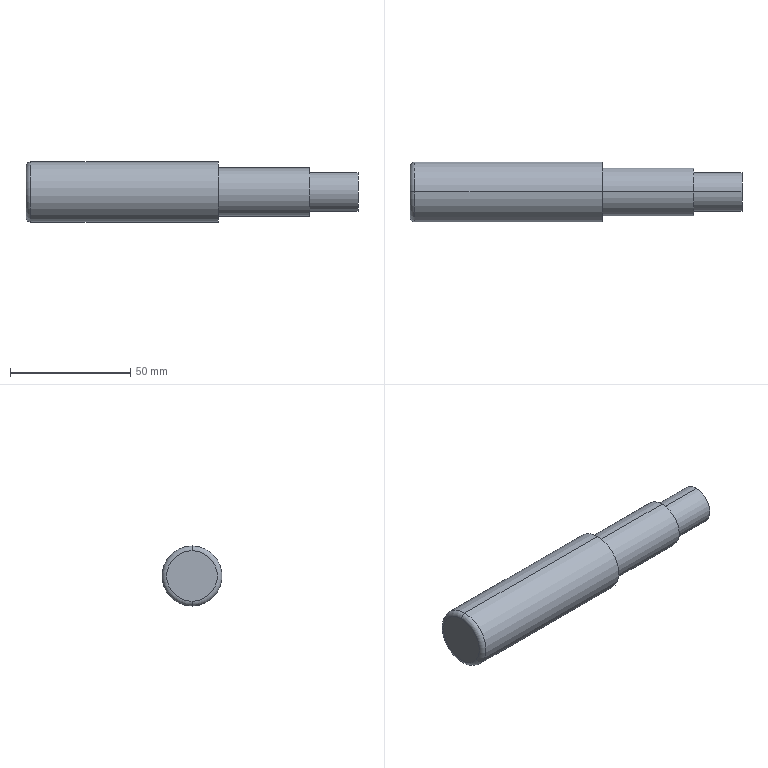Part | SolidWorks | features Fillet 1, Revolution 1 | 1 solid | 12 faces | box 138 x 25 x 25 mm | volume 55164 mm3 | cylinder 6 | plane 4 | torus 2 | commonest cylinder face diameters 16 x2 20 x2 25 x2
STEP:
#1=CARTESIAN_POINT('',(0.,0.,10.5));
#2=VERTEX_POINT('',#1);
#3=CARTESIAN_POINT('',(0.,0.,-10.5));
#4=VERTEX_POINT('',#3);
#5=CARTESIAN_POINT('',(0.,0.,0.));
#6=DIRECTION('',(-1.,0.,0.));
#7=DIRECTION('',(0.,0.,-1.));
#8=AXIS2_PLACEMENT_3D('',#5,#6,#7);
#9=CIRCLE('',#8,10.5);
#10=EDGE_CURVE('',#2,#4,#9,.T.);
#11=ORIENTED_EDGE('',*,*,#10,.F.);
#12=CARTESIAN_POINT('',(2.,0.,12.5));
#13=VERTEX_POINT('',#12);
#14=CARTESIAN_POINT('',(2.,0.,10.5));
#15=DIRECTION('',(0.,1.,0.));
#16=DIRECTION('',(0.,0.,1.));
#17=AXIS2_PLACEMENT_3D('',#14,#15,#16);
#18=CIRCLE('',#17,2.);
#19=EDGE_CURVE('',#2,#13,#18,.T.);
#20=ORIENTED_EDGE('',*,*,#19,.T.);
#21=CARTESIAN_POINT('',(2.,0.,-12.5));
#22=VERTEX_POINT('',#21);
#23=CARTESIAN_POINT('',(2.,0.,0.));
#24=DIRECTION('',(1.,0.,0.));
#25=DIRECTION('',(0.,0.,-1.));
#26=AXIS2_PLACEMENT_3D('',#23,#24,#25);
#27=CIRCLE('',#26,12.5);
#28=EDGE_CURVE('',#22,#13,#27,.T.);
#29=ORIENTED_EDGE('',*,*,#28,.F.);
#30=CARTESIAN_POINT('',(2.,0.,-10.5));
#31=DIRECTION('',(0.,-1.,0.));
#32=DIRECTION('',(0.,0.,-1.));
#33=AXIS2_PLACEMENT_3D('',#30,#31,#32);
#34=CIRCLE('',#33,2.);
#35=EDGE_CURVE('',#4,#22,#34,.T.);
#36=ORIENTED_EDGE('',*,*,#35,.F.);
#37=EDGE_LOOP('',(#11,#20,#29,#36));
#38=FACE_OUTER_BOUND('',#37,.T.);
#39=CARTESIAN_POINT('',(2.,0.,0.));
#40=DIRECTION('',(1.,0.,0.));
#41=DIRECTION('',(0.,0.,-1.));
#42=AXIS2_PLACEMENT_3D('',#39,#40,#41);
#43=TOROIDAL_SURFACE('',#42,10.5,2.);
#44=ADVANCED_FACE('',(#38),#43,.T.);
#45=CARTESIAN_POINT('',(138.,0.,8.));
#46=VERTEX_POINT('',#45);
#47=CARTESIAN_POINT('',(138.,0.,-8.));
#48=VERTEX_POINT('',#47);
#49=CARTESIAN_POINT('',(138.,0.,0.));
#50=DIRECTION('',(-1.,0.,0.));
#51=DIRECTION('',(0.,0.,1.));
#52=AXIS2_PLACEMENT_3D('',#49,#50,#51);
#53=CIRCLE('',#52,8.);
#54=EDGE_CURVE('',#46,#48,#53,.T.);
#55=ORIENTED_EDGE('',*,*,#54,.T.);
#56=CARTESIAN_POINT('',(118.,0.,-8.));
#57=VERTEX_POINT('',#56);
#58=CARTESIAN_POINT('',(0.,0.,-8.));
#59=DIRECTION('',(-1.,0.,0.));
#60=VECTOR('',#59,1000.);
#61=LINE('',#58,#60);
#62=EDGE_CURVE('',#48,#57,#61,.T.);
#63=ORIENTED_EDGE('',*,*,#62,.T.);
#64=CARTESIAN_POINT('',(118.,0.,8.));
#65=VERTEX_POINT('',#64);
#66=CARTESIAN_POINT('',(118.,0.,0.));
#67=DIRECTION('',(-1.,0.,0.));
#68=DIRECTION('',(0.,0.,1.));
#69=AXIS2_PLACEMENT_3D('',#66,#67,#68);
#70=CIRCLE('',#69,8.);
#71=EDGE_CURVE('',#65,#57,#70,.T.);
#72=ORIENTED_EDGE('',*,*,#71,.F.);
#73=CARTESIAN_POINT('',(0.,0.,8.));
#74=DIRECTION('',(-1.,0.,0.));
#75=VECTOR('',#74,1000.);
#76=LINE('',#73,#75);
#77=EDGE_CURVE('',#46,#65,#76,.T.);
#78=ORIENTED_EDGE('',*,*,#77,.F.);
#79=EDGE_LOOP('',(#55,#63,#72,#78));
#80=FACE_OUTER_BOUND('',#79,.T.);
#81=CARTESIAN_POINT('',(0.,0.,0.));
#82=DIRECTION('',(-1.,0.,0.));
#83=DIRECTION('',(0.,0.,1.));
#84=AXIS2_PLACEMENT_3D('',#81,#82,#83);
#85=CYLINDRICAL_SURFACE('',#84,8.);
#86=ADVANCED_FACE('',(#80),#85,.T.);
#87=CARTESIAN_POINT('',(118.,0.,10.));
#88=VERTEX_POINT('',#87);
#89=CARTESIAN_POINT('',(118.,0.,-10.));
#90=VERTEX_POINT('',#89);
#91=CARTESIAN_POINT('',(118.,0.,0.));
#92=DIRECTION('',(-1.,0.,0.));
#93=DIRECTION('',(0.,0.,1.));
#94=AXIS2_PLACEMENT_3D('',#91,#92,#93);
#95=CIRCLE('',#94,10.);
#96=EDGE_CURVE('',#88,#90,#95,.T.);
#97=ORIENTED_EDGE('',*,*,#96,.T.);
#98=CARTESIAN_POINT('',(80.,0.,-10.));
#99=VERTEX_POINT('',#98);
#100=CARTESIAN_POINT('',(0.,0.,-10.));
#101=DIRECTION('',(-1.,0.,0.));
#102=VECTOR('',#101,1000.);
#103=LINE('',#100,#102);
#104=EDGE_CURVE('',#90,#99,#103,.T.);
#105=ORIENTED_EDGE('',*,*,#104,.T.);
#106=CARTESIAN_POINT('',(80.,0.,10.));
#107=VERTEX_POINT('',#106);
#108=CARTESIAN_POINT('',(80.,0.,0.));
#109=DIRECTION('',(-1.,0.,0.));
#110=DIRECTION('',(0.,0.,1.));
#111=AXIS2_PLACEMENT_3D('',#108,#109,#110);
#112=CIRCLE('',#111,10.);
#113=EDGE_CURVE('',#107,#99,#112,.T.);
#114=ORIENTED_EDGE('',*,*,#113,.F.);
#115=CARTESIAN_POINT('',(0.,0.,10.));
#116=DIRECTION('',(-1.,0.,0.));
#117=VECTOR('',#116,1000.);
#118=LINE('',#115,#117);
#119=EDGE_CURVE('',#88,#107,#118,.T.);
#120=ORIENTED_EDGE('',*,*,#119,.F.);
#121=EDGE_LOOP('',(#97,#105,#114,#120));
#122=FACE_OUTER_BOUND('',#121,.T.);
#123=CARTESIAN_POINT('',(0.,0.,0.));
#124=DIRECTION('',(-1.,0.,0.));
#125=DIRECTION('',(0.,0.,1.));
#126=AXIS2_PLACEMENT_3D('',#123,#124,#125);
#127=CYLINDRICAL_SURFACE('',#126,10.);
#128=ADVANCED_FACE('',(#122),#127,.T.);
#129=CARTESIAN_POINT('',(80.,0.,12.5));
#130=VERTEX_POINT('',#129);
#131=CARTESIAN_POINT('',(80.,0.,-12.5));
#132=VERTEX_POINT('',#131);
#133=CARTESIAN_POINT('',(80.,0.,0.));
#134=DIRECTION('',(-1.,0.,0.));
#135=DIRECTION('',(0.,0.,1.));
#136=AXIS2_PLACEMENT_3D('',#133,#134,#135);
#137=CIRCLE('',#136,12.5);
#138=EDGE_CURVE('',#130,#132,#137,.T.);
#139=ORIENTED_EDGE('',*,*,#138,.T.);
#140=CARTESIAN_POINT('',(0.,0.,-12.5));
#141=DIRECTION('',(-1.,0.,0.));
#142=VECTOR('',#141,1000.);
#143=LINE('',#140,#142);
#144=EDGE_CURVE('',#132,#22,#143,.T.);
#145=ORIENTED_EDGE('',*,*,#144,.T.);
#146=ORIENTED_EDGE('',*,*,#28,.T.);
#147=CARTESIAN_POINT('',(0.,0.,12.5));
#148=DIRECTION('',(-1.,0.,0.));
#149=VECTOR('',#148,1000.);
#150=LINE('',#147,#149);
#151=EDGE_CURVE('',#130,#13,#150,.T.);
#152=ORIENTED_EDGE('',*,*,#151,.F.);
#153=EDGE_LOOP('',(#139,#145,#146,#152));
#154=FACE_OUTER_BOUND('',#153,.T.);
#155=CARTESIAN_POINT('',(0.,0.,0.));
#156=DIRECTION('',(-1.,0.,0.));
#157=DIRECTION('',(0.,0.,1.));
#158=AXIS2_PLACEMENT_3D('',#155,#156,#157);
#159=CYLINDRICAL_SURFACE('',#158,12.5);
#160=ADVANCED_FACE('',(#154),#159,.T.);
#161=CARTESIAN_POINT('',(0.,0.,0.));
#162=DIRECTION('',(-1.,0.,0.));
#163=DIRECTION('',(0.,0.,-1.));
#164=AXIS2_PLACEMENT_3D('',#161,#162,#163);
#165=CIRCLE('',#164,10.5);
#166=EDGE_CURVE('',#4,#2,#165,.T.);
#167=ORIENTED_EDGE('',*,*,#166,.T.);
#168=ORIENTED_EDGE('',*,*,#10,.T.);
#169=EDGE_LOOP('',(#167,#168));
#170=FACE_OUTER_BOUND('',#169,.T.);
#171=CARTESIAN_POINT('',(0.,0.,0.));
#172=DIRECTION('',(1.,0.,0.));
#173=DIRECTION('',(0.,0.,-1.));
#174=AXIS2_PLACEMENT_3D('',#171,#172,#173);
#175=PLANE('',#174);
#176=ADVANCED_FACE('',(#170),#175,.F.);
#177=ORIENTED_EDGE('',*,*,#144,.F.);
#178=CARTESIAN_POINT('',(80.,0.,0.));
#179=DIRECTION('',(-1.,0.,0.));
#180=DIRECTION('',(0.,0.,1.));
#181=AXIS2_PLACEMENT_3D('',#178,#179,#180);
#182=CIRCLE('',#181,12.5);
#183=EDGE_CURVE('',#132,#130,#182,.T.);
#184=ORIENTED_EDGE('',*,*,#183,.T.);
#185=ORIENTED_EDGE('',*,*,#151,.T.);
#186=CARTESIAN_POINT('',(2.,0.,0.));
#187=DIRECTION('',(1.,0.,0.));
#188=DIRECTION('',(0.,0.,-1.));
#189=AXIS2_PLACEMENT_3D('',#186,#187,#188);
#190=CIRCLE('',#189,12.5);
#191=EDGE_CURVE('',#13,#22,#190,.T.);
#192=ORIENTED_EDGE('',*,*,#191,.T.);
#193=EDGE_LOOP('',(#177,#184,#185,#192));
#194=FACE_OUTER_BOUND('',#193,.T.);
#195=CARTESIAN_POINT('',(0.,0.,0.));
#196=DIRECTION('',(-1.,0.,0.));
#197=DIRECTION('',(0.,0.,1.));
#198=AXIS2_PLACEMENT_3D('',#195,#196,#197);
#199=CYLINDRICAL_SURFACE('',#198,12.5);
#200=ADVANCED_FACE('',(#194),#199,.T.);
#201=ORIENTED_EDGE('',*,*,#138,.F.);
#202=ORIENTED_EDGE('',*,*,#183,.F.);
#203=EDGE_LOOP('',(#201,#202));
#204=FACE_OUTER_BOUND('',#203,.T.);
#205=ORIENTED_EDGE('',*,*,#113,.T.);
#206=CARTESIAN_POINT('',(80.,0.,0.));
#207=DIRECTION('',(-1.,0.,0.));
#208=DIRECTION('',(0.,0.,1.));
#209=AXIS2_PLACEMENT_3D('',#206,#207,#208);
#210=CIRCLE('',#209,10.);
#211=EDGE_CURVE('',#99,#107,#210,.T.);
#212=ORIENTED_EDGE('',*,*,#211,.T.);
#213=EDGE_LOOP('',(#205,#212));
#214=FACE_BOUND('',#213,.T.);
#215=CARTESIAN_POINT('',(80.,12.5,0.));
#216=DIRECTION('',(-1.,0.,0.));
#217=DIRECTION('',(0.,0.,1.));
#218=AXIS2_PLACEMENT_3D('',#215,#216,#217);
#219=PLANE('',#218);
#220=ADVANCED_FACE('',(#204,#214),#219,.F.);
#221=ORIENTED_EDGE('',*,*,#104,.F.);
#222=CARTESIAN_POINT('',(118.,0.,0.));
#223=DIRECTION('',(-1.,0.,0.));
#224=DIRECTION('',(0.,0.,1.));
#225=AXIS2_PLACEMENT_3D('',#222,#223,#224);
#226=CIRCLE('',#225,10.);
#227=EDGE_CURVE('',#90,#88,#226,.T.);
#228=ORIENTED_EDGE('',*,*,#227,.T.);
#229=ORIENTED_EDGE('',*,*,#119,.T.);
#230=ORIENTED_EDGE('',*,*,#211,.F.);
#231=EDGE_LOOP('',(#221,#228,#229,#230));
#232=FACE_OUTER_BOUND('',#231,.T.);
#233=CARTESIAN_POINT('',(0.,0.,0.));
#234=DIRECTION('',(-1.,0.,0.));
#235=DIRECTION('',(0.,0.,1.));
#236=AXIS2_PLACEMENT_3D('',#233,#234,#235);
#237=CYLINDRICAL_SURFACE('',#236,10.);
#238=ADVANCED_FACE('',(#232),#237,.T.);
#239=ORIENTED_EDGE('',*,*,#96,.F.);
#240=ORIENTED_EDGE('',*,*,#227,.F.);
#241=EDGE_LOOP('',(#239,#240));
#242=FACE_OUTER_BOUND('',#241,.T.);
#243=ORIENTED_EDGE('',*,*,#71,.T.);
#244=CARTESIAN_POINT('',(118.,0.,0.));
#245=DIRECTION('',(-1.,0.,0.));
#246=DIRECTION('',(0.,0.,1.));
#247=AXIS2_PLACEMENT_3D('',#244,#245,#246);
#248=CIRCLE('',#247,8.);
#249=EDGE_CURVE('',#57,#65,#248,.T.);
#250=ORIENTED_EDGE('',*,*,#249,.T.);
#251=EDGE_LOOP('',(#243,#250));
#252=FACE_BOUND('',#251,.T.);
#253=CARTESIAN_POINT('',(118.,10.,0.));
#254=DIRECTION('',(-1.,0.,0.));
#255=DIRECTION('',(0.,0.,1.));
#256=AXIS2_PLACEMENT_3D('',#253,#254,#255);
#257=PLANE('',#256);
#258=ADVANCED_FACE('',(#242,#252),#257,.F.);
#259=ORIENTED_EDGE('',*,*,#62,.F.);
#260=CARTESIAN_POINT('',(138.,0.,0.));
#261=DIRECTION('',(-1.,0.,0.));
#262=DIRECTION('',(0.,0.,1.));
#263=AXIS2_PLACEMENT_3D('',#260,#261,#262);
#264=CIRCLE('',#263,8.);
#265=EDGE_CURVE('',#48,#46,#264,.T.);
#266=ORIENTED_EDGE('',*,*,#265,.T.);
#267=ORIENTED_EDGE('',*,*,#77,.T.);
#268=ORIENTED_EDGE('',*,*,#249,.F.);
#269=EDGE_LOOP('',(#259,#266,#267,#268));
#270=FACE_OUTER_BOUND('',#269,.T.);
#271=CARTESIAN_POINT('',(0.,0.,0.));
#272=DIRECTION('',(-1.,0.,0.));
#273=DIRECTION('',(0.,0.,1.));
#274=AXIS2_PLACEMENT_3D('',#271,#272,#273);
#275=CYLINDRICAL_SURFACE('',#274,8.);
#276=ADVANCED_FACE('',(#270),#275,.T.);
#277=ORIENTED_EDGE('',*,*,#54,.F.);
#278=ORIENTED_EDGE('',*,*,#265,.F.);
#279=EDGE_LOOP('',(#277,#278));
#280=FACE_OUTER_BOUND('',#279,.T.);
#281=CARTESIAN_POINT('',(138.,8.,0.));
#282=DIRECTION('',(-1.,0.,0.));
#283=DIRECTION('',(0.,0.,1.));
#284=AXIS2_PLACEMENT_3D('',#281,#282,#283);
#285=PLANE('',#284);
#286=ADVANCED_FACE('',(#280),#285,.F.);
#287=ORIENTED_EDGE('',*,*,#19,.F.);
#288=ORIENTED_EDGE('',*,*,#166,.F.);
#289=ORIENTED_EDGE('',*,*,#35,.T.);
#290=ORIENTED_EDGE('',*,*,#191,.F.);
#291=EDGE_LOOP('',(#287,#288,#289,#290));
#292=FACE_OUTER_BOUND('',#291,.T.);
#293=CARTESIAN_POINT('',(2.,0.,0.));
#294=DIRECTION('',(1.,0.,0.));
#295=DIRECTION('',(0.,0.,-1.));
#296=AXIS2_PLACEMENT_3D('',#293,#294,#295);
#297=TOROIDAL_SURFACE('',#296,10.5,2.);
#298=ADVANCED_FACE('',(#292),#297,.T.);
#299=CLOSED_SHELL('',(#44,#86,#128,#160,#176,#200,#220,#238,#258,#276,#286,#298));
#300=MANIFOLD_SOLID_BREP('',#299);
#301=CARTESIAN_POINT('',(0.,0.,0.));
#302=DIRECTION('',(0.,0.,1.));
#303=DIRECTION('',(1.,0.,0.));
#304=AXIS2_PLACEMENT_3D('',#301,#302,#303);
#305=(LENGTH_UNIT()NAMED_UNIT(*)SI_UNIT(.MILLI.,.METRE.));
#306=UNCERTAINTY_MEASURE_WITH_UNIT(LENGTH_MEASURE(0.00001),#305,'','');
#307=(NAMED_UNIT(*)PLANE_ANGLE_UNIT()SI_UNIT($,.RADIAN.));
#308=(NAMED_UNIT(*)SI_UNIT($,.STERADIAN.)SOLID_ANGLE_UNIT());
#309=(GEOMETRIC_REPRESENTATION_CONTEXT(3)GLOBAL_UNCERTAINTY_ASSIGNED_CONTEXT((#306))GLOBAL_UNIT_ASSIGNED_CONTEXT((#305,#307,#308))REPRESENTATION_CONTEXT('',''));
#310=ADVANCED_BREP_SHAPE_REPRESENTATION('',(#300,#304),#309);